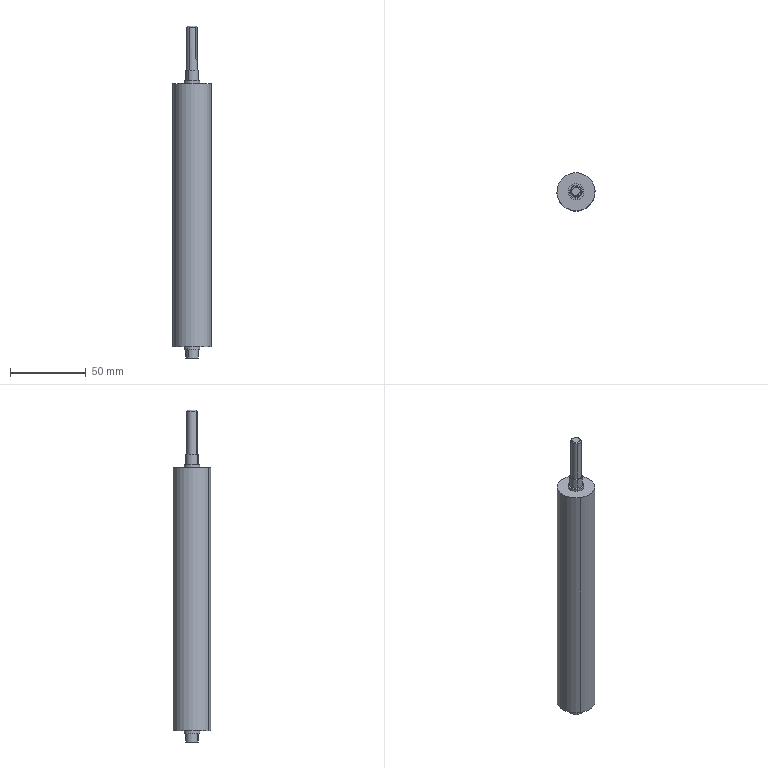Part | SolidWorks | features SplitBody 1 | 1 solid | 27 faces | box 25.2 x 25.2 x 219.8 mm | volume 89003 mm3 | cylinder 14 | plane 10 | cone 3 | commonest cylinder face diameters 8.4 x4 10.5 x4 2.1 x2 7 x2 25.2 x2
STEP:
#1=CARTESIAN_POINT('',(-72.98,240.467,-234.916));
#2=VERTEX_POINT('',#1);
#3=CARTESIAN_POINT('',(-69.853,240.613,-234.916));
#4=VERTEX_POINT('',#3);
#5=CARTESIAN_POINT('',(-71.525,242.859,-234.916));
#6=DIRECTION('',(0.,0.,1.));
#7=DIRECTION('',(-0.5199,-0.8543,0.));
#8=AXIS2_PLACEMENT_3D('',#5,#6,#7);
#9=CIRCLE('',#8,2.8);
#10=EDGE_CURVE('',#2,#4,#9,.T.);
#11=ORIENTED_EDGE('',*,*,#10,.F.);
#12=CARTESIAN_POINT('',(-73.344,239.869,-235.616));
#13=VERTEX_POINT('',#12);
#14=CARTESIAN_POINT('',(-72.98,240.467,-234.916));
#15=DIRECTION('',(-0.3676,-0.604,-0.7071));
#16=VECTOR('',#15,1000.);
#17=LINE('',#14,#16);
#18=EDGE_CURVE('',#2,#13,#17,.T.);
#19=ORIENTED_EDGE('',*,*,#18,.T.);
#20=CARTESIAN_POINT('',(-69.218,240.226,-235.616));
#21=VERTEX_POINT('',#20);
#22=CARTESIAN_POINT('',(-71.525,242.859,-235.616));
#23=DIRECTION('',(0.,0.,-1.));
#24=DIRECTION('',(-0.5199,-0.8543,0.));
#25=AXIS2_PLACEMENT_3D('',#22,#23,#24);
#26=CIRCLE('',#25,3.5);
#27=EDGE_CURVE('',#21,#13,#26,.T.);
#28=ORIENTED_EDGE('',*,*,#27,.F.);
#29=CARTESIAN_POINT('',(-69.853,240.613,-234.916));
#30=CARTESIAN_POINT('',(-69.64,240.483,-235.147));
#31=CARTESIAN_POINT('',(-69.429,240.354,-235.381));
#32=CARTESIAN_POINT('',(-69.218,240.226,-235.616));
#33=B_SPLINE_CURVE_WITH_KNOTS('',3,(#29,#30,#31,#32),.UNSPECIFIED.,.F.,.F.,(4,4),(0.,0.001021),.UNSPECIFIED.);
#34=EDGE_CURVE('',#4,#21,#33,.T.);
#35=ORIENTED_EDGE('',*,*,#34,.F.);
#36=EDGE_LOOP('',(#11,#19,#28,#35));
#37=FACE_OUTER_BOUND('',#36,.T.);
#38=CARTESIAN_POINT('',(-71.525,242.859,-234.916));
#39=DIRECTION('',(0.,0.,-1.));
#40=DIRECTION('',(0.5199,0.8543,0.));
#41=AXIS2_PLACEMENT_3D('',#38,#39,#40);
#42=CONICAL_SURFACE('',#41,2.8,0.7854);
#43=ADVANCED_FACE('',(#37),#42,.T.);
#44=ORIENTED_EDGE('',*,*,#18,.F.);
#45=CARTESIAN_POINT('',(-70.069,245.251,-234.916));
#46=VERTEX_POINT('',#45);
#47=CARTESIAN_POINT('',(-71.525,242.859,-234.916));
#48=DIRECTION('',(0.,0.,1.));
#49=DIRECTION('',(-0.5199,-0.8543,0.));
#50=AXIS2_PLACEMENT_3D('',#47,#48,#49);
#51=CIRCLE('',#50,2.8);
#52=EDGE_CURVE('',#46,#2,#51,.T.);
#53=ORIENTED_EDGE('',*,*,#52,.F.);
#54=CARTESIAN_POINT('',(-69.705,245.849,-235.616));
#55=VERTEX_POINT('',#54);
#56=CARTESIAN_POINT('',(-70.069,245.251,-234.916));
#57=DIRECTION('',(0.3676,0.604,-0.7071));
#58=VECTOR('',#57,1000.);
#59=LINE('',#56,#58);
#60=EDGE_CURVE('',#46,#55,#59,.T.);
#61=ORIENTED_EDGE('',*,*,#60,.T.);
#62=CARTESIAN_POINT('',(-71.525,242.859,-235.616));
#63=DIRECTION('',(0.,0.,-1.));
#64=DIRECTION('',(-0.5199,-0.8543,0.));
#65=AXIS2_PLACEMENT_3D('',#62,#63,#64);
#66=CIRCLE('',#65,3.5);
#67=EDGE_CURVE('',#13,#55,#66,.T.);
#68=ORIENTED_EDGE('',*,*,#67,.F.);
#69=EDGE_LOOP('',(#44,#53,#61,#68));
#70=FACE_OUTER_BOUND('',#69,.T.);
#71=CARTESIAN_POINT('',(-71.525,242.859,-234.916));
#72=DIRECTION('',(0.,0.,-1.));
#73=DIRECTION('',(0.5199,0.8543,0.));
#74=AXIS2_PLACEMENT_3D('',#71,#72,#73);
#75=CONICAL_SURFACE('',#74,2.8,0.7854);
#76=ADVANCED_FACE('',(#70),#75,.T.);
#77=CARTESIAN_POINT('',(-68.535,241.04,-256.966));
#78=VERTEX_POINT('',#77);
#79=CARTESIAN_POINT('',(-69.218,240.226,-255.916));
#80=VERTEX_POINT('',#79);
#81=CARTESIAN_POINT('',(-68.535,241.04,-256.966));
#82=CARTESIAN_POINT('',(-68.606,240.922,-256.966));
#83=CARTESIAN_POINT('',(-68.685,240.809,-256.938));
#84=CARTESIAN_POINT('',(-68.843,240.606,-256.832));
#85=CARTESIAN_POINT('',(-68.921,240.518,-256.755));
#86=CARTESIAN_POINT('',(-69.057,240.375,-256.561));
#87=CARTESIAN_POINT('',(-69.115,240.32,-256.445));
#88=CARTESIAN_POINT('',(-69.196,240.246,-256.193));
#89=CARTESIAN_POINT('',(-69.218,240.226,-256.055));
#90=CARTESIAN_POINT('',(-69.218,240.226,-255.916));
#91=B_SPLINE_CURVE_WITH_KNOTS('',3,(#81,#82,#83,#84,#85,#86,#87,#88,#89,#90),.UNSPECIFIED.,.F.,.F.,(4,2,2,2,4),(0.001651,0.002064,0.002476,0.002888,0.003301),.UNSPECIFIED.);
#92=EDGE_CURVE('',#78,#80,#91,.T.);
#93=ORIENTED_EDGE('',*,*,#92,.F.);
#94=CARTESIAN_POINT('',(-69.671,241.731,-256.966));
#95=VERTEX_POINT('',#94);
#96=CARTESIAN_POINT('',(-60.761,236.309,-256.966));
#97=DIRECTION('',(-0.8543,0.5199,0.));
#98=VECTOR('',#97,1000.);
#99=LINE('',#96,#98);
#100=EDGE_CURVE('',#78,#95,#99,.T.);
#101=ORIENTED_EDGE('',*,*,#100,.T.);
#102=CARTESIAN_POINT('',(-70.217,240.834,-255.916));
#103=VERTEX_POINT('',#102);
#104=CARTESIAN_POINT('',(-69.671,241.731,-255.916));
#105=DIRECTION('',(0.8543,-0.5199,0.));
#106=DIRECTION('',(0.,0.,-1.));
#107=AXIS2_PLACEMENT_3D('',#104,#105,#106);
#108=CIRCLE('',#107,1.05);
#109=EDGE_CURVE('',#103,#95,#108,.T.);
#110=ORIENTED_EDGE('',*,*,#109,.F.);
#111=CARTESIAN_POINT('',(-61.307,235.412,-255.916));
#112=DIRECTION('',(-0.8543,0.5199,0.));
#113=VECTOR('',#112,1000.);
#114=LINE('',#111,#113);
#115=EDGE_CURVE('',#80,#103,#114,.T.);
#116=ORIENTED_EDGE('',*,*,#115,.F.);
#117=EDGE_LOOP('',(#93,#101,#110,#116));
#118=FACE_OUTER_BOUND('',#117,.T.);
#119=CARTESIAN_POINT('',(-60.761,236.309,-255.916));
#120=DIRECTION('',(-0.8543,0.5199,0.));
#121=DIRECTION('',(0.,0.,-1.));
#122=AXIS2_PLACEMENT_3D('',#119,#120,#121);
#123=CYLINDRICAL_SURFACE('',#122,1.05);
#124=ADVANCED_FACE('',(#118),#123,.F.);
#125=CARTESIAN_POINT('',(-69.341,246.447,-454.716));
#126=VERTEX_POINT('',#125);
#127=CARTESIAN_POINT('',(-73.708,239.271,-454.716));
#128=VERTEX_POINT('',#127);
#129=CARTESIAN_POINT('',(-71.525,242.859,-454.716));
#130=DIRECTION('',(0.,0.,-1.));
#131=DIRECTION('',(0.5199,0.8543,0.));
#132=AXIS2_PLACEMENT_3D('',#129,#130,#131);
#133=CIRCLE('',#132,4.2);
#134=EDGE_CURVE('',#126,#128,#133,.T.);
#135=ORIENTED_EDGE('',*,*,#134,.F.);
#136=CARTESIAN_POINT('',(-69.341,246.447,-449.116));
#137=VERTEX_POINT('',#136);
#138=CARTESIAN_POINT('',(-69.341,246.447,-454.716));
#139=DIRECTION('',(0.,0.,1.));
#140=VECTOR('',#139,1000.);
#141=LINE('',#138,#140);
#142=EDGE_CURVE('',#126,#137,#141,.T.);
#143=ORIENTED_EDGE('',*,*,#142,.T.);
#144=CARTESIAN_POINT('',(-73.708,239.271,-449.116));
#145=VERTEX_POINT('',#144);
#146=CARTESIAN_POINT('',(-71.525,242.859,-449.116));
#147=DIRECTION('',(0.,0.,-1.));
#148=DIRECTION('',(0.5199,0.8543,0.));
#149=AXIS2_PLACEMENT_3D('',#146,#147,#148);
#150=CIRCLE('',#149,4.2);
#151=EDGE_CURVE('',#137,#145,#150,.T.);
#152=ORIENTED_EDGE('',*,*,#151,.T.);
#153=CARTESIAN_POINT('',(-73.708,239.271,-454.716));
#154=DIRECTION('',(0.,0.,1.));
#155=VECTOR('',#154,1000.);
#156=LINE('',#153,#155);
#157=EDGE_CURVE('',#128,#145,#156,.T.);
#158=ORIENTED_EDGE('',*,*,#157,.F.);
#159=EDGE_LOOP('',(#135,#143,#152,#158));
#160=FACE_OUTER_BOUND('',#159,.T.);
#161=CARTESIAN_POINT('',(-71.525,242.859,-454.716));
#162=DIRECTION('',(0.,0.,1.));
#163=DIRECTION('',(-0.5199,-0.8543,0.));
#164=AXIS2_PLACEMENT_3D('',#161,#162,#163);
#165=CYLINDRICAL_SURFACE('',#164,4.2);
#166=ADVANCED_FACE('',(#160),#165,.T.);
#167=CARTESIAN_POINT('',(-73.708,239.271,-264.316));
#168=VERTEX_POINT('',#167);
#169=CARTESIAN_POINT('',(-69.341,246.447,-264.316));
#170=VERTEX_POINT('',#169);
#171=CARTESIAN_POINT('',(-71.525,242.859,-264.316));
#172=DIRECTION('',(0.,0.,1.));
#173=DIRECTION('',(-0.5199,-0.8543,0.));
#174=AXIS2_PLACEMENT_3D('',#171,#172,#173);
#175=CIRCLE('',#174,4.2);
#176=EDGE_CURVE('',#168,#170,#175,.T.);
#177=ORIENTED_EDGE('',*,*,#176,.F.);
#178=CARTESIAN_POINT('',(-73.708,239.271,-271.316));
#179=VERTEX_POINT('',#178);
#180=CARTESIAN_POINT('',(-73.708,239.271,-264.316));
#181=DIRECTION('',(0.,0.,-1.));
#182=VECTOR('',#181,1000.);
#183=LINE('',#180,#182);
#184=EDGE_CURVE('',#168,#179,#183,.T.);
#185=ORIENTED_EDGE('',*,*,#184,.T.);
#186=CARTESIAN_POINT('',(-69.341,246.447,-271.316));
#187=VERTEX_POINT('',#186);
#188=CARTESIAN_POINT('',(-71.525,242.859,-271.316));
#189=DIRECTION('',(0.,0.,1.));
#190=DIRECTION('',(-0.5199,-0.8543,0.));
#191=AXIS2_PLACEMENT_3D('',#188,#189,#190);
#192=CIRCLE('',#191,4.2);
#193=EDGE_CURVE('',#179,#187,#192,.T.);
#194=ORIENTED_EDGE('',*,*,#193,.T.);
#195=CARTESIAN_POINT('',(-69.341,246.447,-264.316));
#196=DIRECTION('',(0.,0.,-1.));
#197=VECTOR('',#196,1000.);
#198=LINE('',#195,#197);
#199=EDGE_CURVE('',#170,#187,#198,.T.);
#200=ORIENTED_EDGE('',*,*,#199,.F.);
#201=EDGE_LOOP('',(#177,#185,#194,#200));
#202=FACE_OUTER_BOUND('',#201,.T.);
#203=CARTESIAN_POINT('',(-71.525,242.859,-264.316));
#204=DIRECTION('',(0.,0.,-1.));
#205=DIRECTION('',(0.5199,0.8543,0.));
#206=AXIS2_PLACEMENT_3D('',#203,#204,#205);
#207=CYLINDRICAL_SURFACE('',#206,4.2);
#208=ADVANCED_FACE('',(#202),#207,.T.);
#209=CARTESIAN_POINT('',(-68.795,247.344,-449.116));
#210=VERTEX_POINT('',#209);
#211=CARTESIAN_POINT('',(-74.254,238.374,-449.116));
#212=VERTEX_POINT('',#211);
#213=CARTESIAN_POINT('',(-71.525,242.859,-449.116));
#214=DIRECTION('',(0.,0.,-1.));
#215=DIRECTION('',(0.5199,0.8543,0.));
#216=AXIS2_PLACEMENT_3D('',#213,#214,#215);
#217=CIRCLE('',#216,5.25);
#218=EDGE_CURVE('',#210,#212,#217,.T.);
#219=ORIENTED_EDGE('',*,*,#218,.F.);
#220=CARTESIAN_POINT('',(-68.795,247.344,-447.366));
#221=VERTEX_POINT('',#220);
#222=CARTESIAN_POINT('',(-68.795,247.344,-449.116));
#223=DIRECTION('',(0.,0.,1.));
#224=VECTOR('',#223,1000.);
#225=LINE('',#222,#224);
#226=EDGE_CURVE('',#210,#221,#225,.T.);
#227=ORIENTED_EDGE('',*,*,#226,.T.);
#228=CARTESIAN_POINT('',(-74.254,238.374,-447.366));
#229=VERTEX_POINT('',#228);
#230=CARTESIAN_POINT('',(-71.525,242.859,-447.366));
#231=DIRECTION('',(0.,0.,-1.));
#232=DIRECTION('',(-0.5199,-0.8543,0.));
#233=AXIS2_PLACEMENT_3D('',#230,#231,#232);
#234=CIRCLE('',#233,5.25);
#235=EDGE_CURVE('',#221,#229,#234,.T.);
#236=ORIENTED_EDGE('',*,*,#235,.T.);
#237=CARTESIAN_POINT('',(-74.254,238.374,-449.116));
#238=DIRECTION('',(0.,0.,1.));
#239=VECTOR('',#238,1000.);
#240=LINE('',#237,#239);
#241=EDGE_CURVE('',#212,#229,#240,.T.);
#242=ORIENTED_EDGE('',*,*,#241,.F.);
#243=EDGE_LOOP('',(#219,#227,#236,#242));
#244=FACE_OUTER_BOUND('',#243,.T.);
#245=CARTESIAN_POINT('',(-71.525,242.859,-449.116));
#246=DIRECTION('',(0.,0.,1.));
#247=DIRECTION('',(-0.5199,-0.8543,0.));
#248=AXIS2_PLACEMENT_3D('',#245,#246,#247);
#249=CYLINDRICAL_SURFACE('',#248,5.25);
#250=ADVANCED_FACE('',(#244),#249,.T.);
#251=CARTESIAN_POINT('',(-74.254,238.374,-271.316));
#252=VERTEX_POINT('',#251);
#253=CARTESIAN_POINT('',(-68.795,247.344,-271.316));
#254=VERTEX_POINT('',#253);
#255=CARTESIAN_POINT('',(-71.525,242.859,-271.316));
#256=DIRECTION('',(0.,0.,1.));
#257=DIRECTION('',(-0.5199,-0.8543,0.));
#258=AXIS2_PLACEMENT_3D('',#255,#256,#257);
#259=CIRCLE('',#258,5.25);
#260=EDGE_CURVE('',#252,#254,#259,.T.);
#261=ORIENTED_EDGE('',*,*,#260,.F.);
#262=CARTESIAN_POINT('',(-74.254,238.374,-273.066));
#263=VERTEX_POINT('',#262);
#264=CARTESIAN_POINT('',(-74.254,238.374,-271.316));
#265=DIRECTION('',(0.,0.,-1.));
#266=VECTOR('',#265,1000.);
#267=LINE('',#264,#266);
#268=EDGE_CURVE('',#252,#263,#267,.T.);
#269=ORIENTED_EDGE('',*,*,#268,.T.);
#270=CARTESIAN_POINT('',(-68.795,247.344,-273.066));
#271=VERTEX_POINT('',#270);
#272=CARTESIAN_POINT('',(-71.525,242.859,-273.066));
#273=DIRECTION('',(0.,0.,1.));
#274=DIRECTION('',(-0.5199,-0.8543,0.));
#275=AXIS2_PLACEMENT_3D('',#272,#273,#274);
#276=CIRCLE('',#275,5.25);
#277=EDGE_CURVE('',#263,#271,#276,.T.);
#278=ORIENTED_EDGE('',*,*,#277,.T.);
#279=CARTESIAN_POINT('',(-68.795,247.344,-271.316));
#280=DIRECTION('',(0.,0.,-1.));
#281=VECTOR('',#280,1000.);
#282=LINE('',#279,#281);
#283=EDGE_CURVE('',#254,#271,#282,.T.);
#284=ORIENTED_EDGE('',*,*,#283,.F.);
#285=EDGE_LOOP('',(#261,#269,#278,#284));
#286=FACE_OUTER_BOUND('',#285,.T.);
#287=CARTESIAN_POINT('',(-71.525,242.859,-271.316));
#288=DIRECTION('',(0.,0.,-1.));
#289=DIRECTION('',(0.5199,0.8543,0.));
#290=AXIS2_PLACEMENT_3D('',#287,#288,#289);
#291=CYLINDRICAL_SURFACE('',#290,5.25);
#292=ADVANCED_FACE('',(#286),#291,.T.);
#293=CARTESIAN_POINT('',(-78.075,232.095,-273.066));
#294=VERTEX_POINT('',#293);
#295=CARTESIAN_POINT('',(-64.975,253.623,-273.066));
#296=VERTEX_POINT('',#295);
#297=CARTESIAN_POINT('',(-71.525,242.859,-273.066));
#298=DIRECTION('',(0.,0.,1.));
#299=DIRECTION('',(-0.5199,-0.8543,0.));
#300=AXIS2_PLACEMENT_3D('',#297,#298,#299);
#301=CIRCLE('',#300,12.6);
#302=EDGE_CURVE('',#294,#296,#301,.T.);
#303=ORIENTED_EDGE('',*,*,#302,.F.);
#304=CARTESIAN_POINT('',(-78.075,232.095,-447.366));
#305=VERTEX_POINT('',#304);
#306=CARTESIAN_POINT('',(-78.075,232.095,-273.066));
#307=DIRECTION('',(0.,0.,-1.));
#308=VECTOR('',#307,1000.);
#309=LINE('',#306,#308);
#310=EDGE_CURVE('',#294,#305,#309,.T.);
#311=ORIENTED_EDGE('',*,*,#310,.T.);
#312=CARTESIAN_POINT('',(-64.975,253.623,-447.366));
#313=VERTEX_POINT('',#312);
#314=CARTESIAN_POINT('',(-71.525,242.859,-447.366));
#315=DIRECTION('',(0.,0.,1.));
#316=DIRECTION('',(-0.5199,-0.8543,0.));
#317=AXIS2_PLACEMENT_3D('',#314,#315,#316);
#318=CIRCLE('',#317,12.6);
#319=EDGE_CURVE('',#305,#313,#318,.T.);
#320=ORIENTED_EDGE('',*,*,#319,.T.);
#321=CARTESIAN_POINT('',(-64.975,253.623,-273.066));
#322=DIRECTION('',(0.,0.,-1.));
#323=VECTOR('',#322,1000.);
#324=LINE('',#321,#323);
#325=EDGE_CURVE('',#296,#313,#324,.T.);
#326=ORIENTED_EDGE('',*,*,#325,.F.);
#327=EDGE_LOOP('',(#303,#311,#320,#326));
#328=FACE_OUTER_BOUND('',#327,.T.);
#329=CARTESIAN_POINT('',(-71.525,242.859,-273.066));
#330=DIRECTION('',(0.,0.,-1.));
#331=DIRECTION('',(0.5199,0.8543,0.));
#332=AXIS2_PLACEMENT_3D('',#329,#330,#331);
#333=CYLINDRICAL_SURFACE('',#332,12.6);
#334=ADVANCED_FACE('',(#328),#333,.T.);
#335=ORIENTED_EDGE('',*,*,#27,.T.);
#336=CARTESIAN_POINT('',(-73.344,239.869,-264.316));
#337=VERTEX_POINT('',#336);
#338=CARTESIAN_POINT('',(-73.344,239.869,-241.916));
#339=DIRECTION('',(0.,0.,-1.));
#340=VECTOR('',#339,1000.);
#341=LINE('',#338,#340);
#342=EDGE_CURVE('',#13,#337,#341,.T.);
#343=ORIENTED_EDGE('',*,*,#342,.T.);
#344=CARTESIAN_POINT('',(-69.705,245.849,-264.316));
#345=VERTEX_POINT('',#344);
#346=CARTESIAN_POINT('',(-71.525,242.859,-264.316));
#347=DIRECTION('',(0.,0.,1.));
#348=DIRECTION('',(-0.5199,-0.8543,0.));
#349=AXIS2_PLACEMENT_3D('',#346,#347,#348);
#350=CIRCLE('',#349,3.5);
#351=EDGE_CURVE('',#337,#345,#350,.T.);
#352=ORIENTED_EDGE('',*,*,#351,.T.);
#353=CARTESIAN_POINT('',(-69.705,245.849,-241.916));
#354=DIRECTION('',(0.,0.,-1.));
#355=VECTOR('',#354,1000.);
#356=LINE('',#353,#355);
#357=EDGE_CURVE('',#55,#345,#356,.T.);
#358=ORIENTED_EDGE('',*,*,#357,.F.);
#359=CARTESIAN_POINT('',(-68.127,242.02,-235.616));
#360=VERTEX_POINT('',#359);
#361=CARTESIAN_POINT('',(-71.525,242.859,-235.616));
#362=DIRECTION('',(0.,0.,-1.));
#363=DIRECTION('',(-0.5199,-0.8543,0.));
#364=AXIS2_PLACEMENT_3D('',#361,#362,#363);
#365=CIRCLE('',#364,3.5);
#366=EDGE_CURVE('',#55,#360,#365,.T.);
#367=ORIENTED_EDGE('',*,*,#366,.T.);
#368=CARTESIAN_POINT('',(-68.127,242.02,-255.916));
#369=VERTEX_POINT('',#368);
#370=CARTESIAN_POINT('',(-68.127,242.02,-241.916));
#371=DIRECTION('',(0.,0.,-1.));
#372=VECTOR('',#371,1000.);
#373=LINE('',#370,#372);
#374=EDGE_CURVE('',#360,#369,#373,.T.);
#375=ORIENTED_EDGE('',*,*,#374,.T.);
#376=CARTESIAN_POINT('',(-68.127,242.02,-255.916));
#377=CARTESIAN_POINT('',(-68.127,242.02,-256.055));
#378=CARTESIAN_POINT('',(-68.133,241.992,-256.192));
#379=CARTESIAN_POINT('',(-68.162,241.886,-256.446));
#380=CARTESIAN_POINT('',(-68.185,241.808,-256.562));
#381=CARTESIAN_POINT('',(-68.249,241.622,-256.755));
#382=CARTESIAN_POINT('',(-68.292,241.511,-256.833));
#383=CARTESIAN_POINT('',(-68.398,241.28,-256.938));
#384=CARTESIAN_POINT('',(-68.463,241.157,-256.966));
#385=CARTESIAN_POINT('',(-68.535,241.04,-256.966));
#386=B_SPLINE_CURVE_WITH_KNOTS('',3,(#376,#377,#378,#379,#380,#381,#382,#383,#384,#385),.UNSPECIFIED.,.F.,.F.,(4,2,2,2,4),(0.,0.0004128,0.0008257,0.001239,0.001651),.UNSPECIFIED.);
#387=EDGE_CURVE('',#369,#78,#386,.T.);
#388=ORIENTED_EDGE('',*,*,#387,.T.);
#389=ORIENTED_EDGE('',*,*,#92,.T.);
#390=CARTESIAN_POINT('',(-69.218,240.226,-241.916));
#391=DIRECTION('',(0.,0.,1.));
#392=VECTOR('',#391,1000.);
#393=LINE('',#390,#392);
#394=EDGE_CURVE('',#80,#21,#393,.T.);
#395=ORIENTED_EDGE('',*,*,#394,.T.);
#396=EDGE_LOOP('',(#335,#343,#352,#358,#367,#375,#388,#389,#395));
#397=FACE_OUTER_BOUND('',#396,.T.);
#398=CARTESIAN_POINT('',(-71.525,242.859,-241.916));
#399=DIRECTION('',(0.,0.,-1.));
#400=DIRECTION('',(0.5199,0.8543,0.));
#401=AXIS2_PLACEMENT_3D('',#398,#399,#400);
#402=CYLINDRICAL_SURFACE('',#401,3.5);
#403=ADVANCED_FACE('',(#397),#402,.T.);
#404=ORIENTED_EDGE('',*,*,#342,.F.);
#405=ORIENTED_EDGE('',*,*,#67,.T.);
#406=ORIENTED_EDGE('',*,*,#357,.T.);
#407=CARTESIAN_POINT('',(-71.525,242.859,-264.316));
#408=DIRECTION('',(0.,0.,1.));
#409=DIRECTION('',(-0.5199,-0.8543,0.));
#410=AXIS2_PLACEMENT_3D('',#407,#408,#409);
#411=CIRCLE('',#410,3.5);
#412=EDGE_CURVE('',#345,#337,#411,.T.);
#413=ORIENTED_EDGE('',*,*,#412,.T.);
#414=EDGE_LOOP('',(#404,#405,#406,#413));
#415=FACE_OUTER_BOUND('',#414,.T.);
#416=CARTESIAN_POINT('',(-71.525,242.859,-241.916));
#417=DIRECTION('',(0.,0.,-1.));
#418=DIRECTION('',(0.5199,0.8543,0.));
#419=AXIS2_PLACEMENT_3D('',#416,#417,#418);
#420=CYLINDRICAL_SURFACE('',#419,3.5);
#421=ADVANCED_FACE('',(#415),#420,.T.);
#422=CARTESIAN_POINT('',(-71.525,242.859,-449.116));
#423=DIRECTION('',(0.,0.,-1.));
#424=DIRECTION('',(0.5199,0.8543,0.));
#425=AXIS2_PLACEMENT_3D('',#422,#423,#424);
#426=CIRCLE('',#425,5.25);
#427=EDGE_CURVE('',#212,#210,#426,.T.);
#428=ORIENTED_EDGE('',*,*,#427,.T.);
#429=ORIENTED_EDGE('',*,*,#218,.T.);
#430=EDGE_LOOP('',(#428,#429));
#431=FACE_OUTER_BOUND('',#430,.T.);
#432=CARTESIAN_POINT('',(-71.525,242.859,-449.116));
#433=DIRECTION('',(0.,0.,-1.));
#434=DIRECTION('',(0.5199,0.8543,0.));
#435=AXIS2_PLACEMENT_3D('',#432,#433,#434);
#436=CIRCLE('',#435,4.2);
#437=EDGE_CURVE('',#145,#137,#436,.T.);
#438=ORIENTED_EDGE('',*,*,#437,.F.);
#439=ORIENTED_EDGE('',*,*,#151,.F.);
#440=EDGE_LOOP('',(#438,#439));
#441=FACE_BOUND('',#440,.T.);
#442=CARTESIAN_POINT('',(-71.525,242.859,-449.116));
#443=DIRECTION('',(0.,0.,-1.));
#444=DIRECTION('',(0.5199,0.8543,0.));
#445=AXIS2_PLACEMENT_3D('',#442,#443,#444);
#446=PLANE('',#445);
#447=ADVANCED_FACE('',(#431,#441),#446,.T.);
#448=CARTESIAN_POINT('',(-71.525,242.859,-271.316));
#449=DIRECTION('',(0.,0.,1.));
#450=DIRECTION('',(-0.5199,-0.8543,0.));
#451=AXIS2_PLACEMENT_3D('',#448,#449,#450);
#452=CIRCLE('',#451,5.25);
#453=EDGE_CURVE('',#254,#252,#452,.T.);
#454=ORIENTED_EDGE('',*,*,#453,.T.);
#455=ORIENTED_EDGE('',*,*,#260,.T.);
#456=EDGE_LOOP('',(#454,#455));
#457=FACE_OUTER_BOUND('',#456,.T.);
#458=CARTESIAN_POINT('',(-71.525,242.859,-271.316));
#459=DIRECTION('',(0.,0.,1.));
#460=DIRECTION('',(-0.5199,-0.8543,0.));
#461=AXIS2_PLACEMENT_3D('',#458,#459,#460);
#462=CIRCLE('',#461,4.2);
#463=EDGE_CURVE('',#187,#179,#462,.T.);
#464=ORIENTED_EDGE('',*,*,#463,.F.);
#465=ORIENTED_EDGE('',*,*,#193,.F.);
#466=EDGE_LOOP('',(#464,#465));
#467=FACE_BOUND('',#466,.T.);
#468=CARTESIAN_POINT('',(-71.525,242.859,-271.316));
#469=DIRECTION('',(0.,0.,1.));
#470=DIRECTION('',(-0.5199,-0.8543,0.));
#471=AXIS2_PLACEMENT_3D('',#468,#469,#470);
#472=PLANE('',#471);
#473=ADVANCED_FACE('',(#457,#467),#472,.T.);
#474=CARTESIAN_POINT('',(-71.525,242.859,-447.366));
#475=DIRECTION('',(0.,0.,1.));
#476=DIRECTION('',(-0.5199,-0.8543,0.));
#477=AXIS2_PLACEMENT_3D('',#474,#475,#476);
#478=CIRCLE('',#477,12.6);
#479=EDGE_CURVE('',#313,#305,#478,.T.);
#480=ORIENTED_EDGE('',*,*,#479,.F.);
#481=ORIENTED_EDGE('',*,*,#319,.F.);
#482=EDGE_LOOP('',(#480,#481));
#483=FACE_OUTER_BOUND('',#482,.T.);
#484=CARTESIAN_POINT('',(-71.525,242.859,-447.366));
#485=DIRECTION('',(0.,0.,-1.));
#486=DIRECTION('',(-0.5199,-0.8543,0.));
#487=AXIS2_PLACEMENT_3D('',#484,#485,#486);
#488=CIRCLE('',#487,5.25);
#489=EDGE_CURVE('',#229,#221,#488,.T.);
#490=ORIENTED_EDGE('',*,*,#489,.F.);
#491=ORIENTED_EDGE('',*,*,#235,.F.);
#492=EDGE_LOOP('',(#490,#491));
#493=FACE_BOUND('',#492,.T.);
#494=CARTESIAN_POINT('',(-71.525,242.859,-447.366));
#495=DIRECTION('',(0.,0.,1.));
#496=DIRECTION('',(-0.5199,-0.8543,0.));
#497=AXIS2_PLACEMENT_3D('',#494,#495,#496);
#498=PLANE('',#497);
#499=ADVANCED_FACE('',(#483,#493),#498,.F.);
#500=CARTESIAN_POINT('',(-71.525,242.859,-273.066));
#501=DIRECTION('',(0.,0.,1.));
#502=DIRECTION('',(-0.5199,-0.8543,0.));
#503=AXIS2_PLACEMENT_3D('',#500,#501,#502);
#504=CIRCLE('',#503,12.6);
#505=EDGE_CURVE('',#296,#294,#504,.T.);
#506=ORIENTED_EDGE('',*,*,#505,.T.);
#507=ORIENTED_EDGE('',*,*,#302,.T.);
#508=EDGE_LOOP('',(#506,#507));
#509=FACE_OUTER_BOUND('',#508,.T.);
#510=CARTESIAN_POINT('',(-71.525,242.859,-273.066));
#511=DIRECTION('',(0.,0.,1.));
#512=DIRECTION('',(-0.5199,-0.8543,0.));
#513=AXIS2_PLACEMENT_3D('',#510,#511,#512);
#514=CIRCLE('',#513,5.25);
#515=EDGE_CURVE('',#271,#263,#514,.T.);
#516=ORIENTED_EDGE('',*,*,#515,.F.);
#517=ORIENTED_EDGE('',*,*,#277,.F.);
#518=EDGE_LOOP('',(#516,#517));
#519=FACE_BOUND('',#518,.T.);
#520=CARTESIAN_POINT('',(-71.525,242.859,-273.066));
#521=DIRECTION('',(0.,0.,1.));
#522=DIRECTION('',(-0.5199,-0.8543,0.));
#523=AXIS2_PLACEMENT_3D('',#520,#521,#522);
#524=PLANE('',#523);
#525=ADVANCED_FACE('',(#509,#519),#524,.T.);
#526=ORIENTED_EDGE('',*,*,#310,.F.);
#527=ORIENTED_EDGE('',*,*,#505,.F.);
#528=ORIENTED_EDGE('',*,*,#325,.T.);
#529=ORIENTED_EDGE('',*,*,#479,.T.);
#530=EDGE_LOOP('',(#526,#527,#528,#529));
#531=FACE_OUTER_BOUND('',#530,.T.);
#532=CARTESIAN_POINT('',(-71.525,242.859,-273.066));
#533=DIRECTION('',(0.,0.,-1.));
#534=DIRECTION('',(0.5199,0.8543,0.));
#535=AXIS2_PLACEMENT_3D('',#532,#533,#534);
#536=CYLINDRICAL_SURFACE('',#535,12.6);
#537=ADVANCED_FACE('',(#531),#536,.T.);
#538=ORIENTED_EDGE('',*,*,#268,.F.);
#539=ORIENTED_EDGE('',*,*,#453,.F.);
#540=ORIENTED_EDGE('',*,*,#283,.T.);
#541=ORIENTED_EDGE('',*,*,#515,.T.);
#542=EDGE_LOOP('',(#538,#539,#540,#541));
#543=FACE_OUTER_BOUND('',#542,.T.);
#544=CARTESIAN_POINT('',(-71.525,242.859,-271.316));
#545=DIRECTION('',(0.,0.,-1.));
#546=DIRECTION('',(0.5199,0.8543,0.));
#547=AXIS2_PLACEMENT_3D('',#544,#545,#546);
#548=CYLINDRICAL_SURFACE('',#547,5.25);
#549=ADVANCED_FACE('',(#543),#548,.T.);
#550=ORIENTED_EDGE('',*,*,#226,.F.);
#551=ORIENTED_EDGE('',*,*,#427,.F.);
#552=ORIENTED_EDGE('',*,*,#241,.T.);
#553=ORIENTED_EDGE('',*,*,#489,.T.);
#554=EDGE_LOOP('',(#550,#551,#552,#553));
#555=FACE_OUTER_BOUND('',#554,.T.);
#556=CARTESIAN_POINT('',(-71.525,242.859,-449.116));
#557=DIRECTION('',(0.,0.,1.));
#558=DIRECTION('',(-0.5199,-0.8543,0.));
#559=AXIS2_PLACEMENT_3D('',#556,#557,#558);
#560=CYLINDRICAL_SURFACE('',#559,5.25);
#561=ADVANCED_FACE('',(#555),#560,.T.);
#562=ORIENTED_EDGE('',*,*,#184,.F.);
#563=CARTESIAN_POINT('',(-71.525,242.859,-264.316));
#564=DIRECTION('',(0.,0.,1.));
#565=DIRECTION('',(-0.5199,-0.8543,0.));
#566=AXIS2_PLACEMENT_3D('',#563,#564,#565);
#567=CIRCLE('',#566,4.2);
#568=EDGE_CURVE('',#170,#168,#567,.T.);
#569=ORIENTED_EDGE('',*,*,#568,.F.);
#570=ORIENTED_EDGE('',*,*,#199,.T.);
#571=ORIENTED_EDGE('',*,*,#463,.T.);
#572=EDGE_LOOP('',(#562,#569,#570,#571));
#573=FACE_OUTER_BOUND('',#572,.T.);
#574=CARTESIAN_POINT('',(-71.525,242.859,-264.316));
#575=DIRECTION('',(0.,0.,-1.));
#576=DIRECTION('',(0.5199,0.8543,0.));
#577=AXIS2_PLACEMENT_3D('',#574,#575,#576);
#578=CYLINDRICAL_SURFACE('',#577,4.2);
#579=ADVANCED_FACE('',(#573),#578,.T.);
#580=ORIENTED_EDGE('',*,*,#412,.F.);
#581=ORIENTED_EDGE('',*,*,#351,.F.);
#582=EDGE_LOOP('',(#580,#581));
#583=FACE_BOUND('',#582,.T.);
#584=ORIENTED_EDGE('',*,*,#568,.T.);
#585=ORIENTED_EDGE('',*,*,#176,.T.);
#586=EDGE_LOOP('',(#584,#585));
#587=FACE_OUTER_BOUND('',#586,.T.);
#588=CARTESIAN_POINT('',(-71.525,242.859,-264.316));
#589=DIRECTION('',(0.,0.,1.));
#590=DIRECTION('',(-0.5199,-0.8543,0.));
#591=AXIS2_PLACEMENT_3D('',#588,#589,#590);
#592=PLANE('',#591);
#593=ADVANCED_FACE('',(#583,#587),#592,.T.);
#594=ORIENTED_EDGE('',*,*,#142,.F.);
#595=CARTESIAN_POINT('',(-71.525,242.859,-454.716));
#596=DIRECTION('',(0.,0.,-1.));
#597=DIRECTION('',(0.5199,0.8543,0.));
#598=AXIS2_PLACEMENT_3D('',#595,#596,#597);
#599=CIRCLE('',#598,4.2);
#600=EDGE_CURVE('',#128,#126,#599,.T.);
#601=ORIENTED_EDGE('',*,*,#600,.F.);
#602=ORIENTED_EDGE('',*,*,#157,.T.);
#603=ORIENTED_EDGE('',*,*,#437,.T.);
#604=EDGE_LOOP('',(#594,#601,#602,#603));
#605=FACE_OUTER_BOUND('',#604,.T.);
#606=CARTESIAN_POINT('',(-71.525,242.859,-454.716));
#607=DIRECTION('',(0.,0.,1.));
#608=DIRECTION('',(-0.5199,-0.8543,0.));
#609=AXIS2_PLACEMENT_3D('',#606,#607,#608);
#610=CYLINDRICAL_SURFACE('',#609,4.2);
#611=ADVANCED_FACE('',(#605),#610,.T.);
#612=ORIENTED_EDGE('',*,*,#600,.T.);
#613=ORIENTED_EDGE('',*,*,#134,.T.);
#614=EDGE_LOOP('',(#612,#613));
#615=FACE_OUTER_BOUND('',#614,.T.);
#616=CARTESIAN_POINT('',(-71.525,242.859,-454.716));
#617=DIRECTION('',(0.,0.,-1.));
#618=DIRECTION('',(0.5199,0.8543,0.));
#619=AXIS2_PLACEMENT_3D('',#616,#617,#618);
#620=PLANE('',#619);
#621=ADVANCED_FACE('',(#615),#620,.T.);
#622=CARTESIAN_POINT('',(-70.217,240.834,-234.916));
#623=VERTEX_POINT('',#622);
#624=CARTESIAN_POINT('',(-70.217,240.834,-234.916));
#625=DIRECTION('',(-0.8543,0.5199,0.));
#626=VECTOR('',#625,1000.);
#627=LINE('',#624,#626);
#628=EDGE_CURVE('',#4,#623,#627,.T.);
#629=ORIENTED_EDGE('',*,*,#628,.F.);
#630=ORIENTED_EDGE('',*,*,#34,.T.);
#631=ORIENTED_EDGE('',*,*,#394,.F.);
#632=ORIENTED_EDGE('',*,*,#115,.T.);
#633=CARTESIAN_POINT('',(-70.217,240.834,-255.916));
#634=DIRECTION('',(0.,0.,-1.));
#635=VECTOR('',#634,1000.);
#636=LINE('',#633,#635);
#637=EDGE_CURVE('',#623,#103,#636,.T.);
#638=ORIENTED_EDGE('',*,*,#637,.F.);
#639=EDGE_LOOP('',(#629,#630,#631,#632,#638));
#640=FACE_OUTER_BOUND('',#639,.T.);
#641=CARTESIAN_POINT('',(-61.307,235.412,-255.916));
#642=DIRECTION('',(0.5199,0.8543,0.));
#643=DIRECTION('',(0.,0.,1.));
#644=AXIS2_PLACEMENT_3D('',#641,#642,#643);
#645=PLANE('',#644);
#646=ADVANCED_FACE('',(#640),#645,.T.);
#647=ORIENTED_EDGE('',*,*,#100,.F.);
#648=ORIENTED_EDGE('',*,*,#387,.F.);
#649=CARTESIAN_POINT('',(-69.125,242.628,-255.916));
#650=VERTEX_POINT('',#649);
#651=CARTESIAN_POINT('',(-60.215,237.206,-255.916));
#652=DIRECTION('',(-0.8543,0.5199,0.));
#653=VECTOR('',#652,1000.);
#654=LINE('',#651,#653);
#655=EDGE_CURVE('',#369,#650,#654,.T.);
#656=ORIENTED_EDGE('',*,*,#655,.T.);
#657=CARTESIAN_POINT('',(-69.671,241.731,-255.916));
#658=DIRECTION('',(0.8543,-0.5199,0.));
#659=DIRECTION('',(0.,0.,-1.));
#660=AXIS2_PLACEMENT_3D('',#657,#658,#659);
#661=CIRCLE('',#660,1.05);
#662=EDGE_CURVE('',#95,#650,#661,.T.);
#663=ORIENTED_EDGE('',*,*,#662,.F.);
#664=EDGE_LOOP('',(#647,#648,#656,#663));
#665=FACE_OUTER_BOUND('',#664,.T.);
#666=CARTESIAN_POINT('',(-60.761,236.309,-255.916));
#667=DIRECTION('',(-0.8543,0.5199,0.));
#668=DIRECTION('',(0.,0.,-1.));
#669=AXIS2_PLACEMENT_3D('',#666,#667,#668);
#670=CYLINDRICAL_SURFACE('',#669,1.05);
#671=ADVANCED_FACE('',(#665),#670,.F.);
#672=ORIENTED_EDGE('',*,*,#374,.F.);
#673=CARTESIAN_POINT('',(-68.761,242.407,-234.916));
#674=VERTEX_POINT('',#673);
#675=CARTESIAN_POINT('',(-68.127,242.02,-235.616));
#676=CARTESIAN_POINT('',(-68.337,242.148,-235.381));
#677=CARTESIAN_POINT('',(-68.548,242.277,-235.147));
#678=CARTESIAN_POINT('',(-68.761,242.407,-234.916));
#679=B_SPLINE_CURVE_WITH_KNOTS('',3,(#675,#676,#677,#678),.UNSPECIFIED.,.F.,.F.,(4,4),(0.,0.001021),.UNSPECIFIED.);
#680=EDGE_CURVE('',#360,#674,#679,.T.);
#681=ORIENTED_EDGE('',*,*,#680,.T.);
#682=CARTESIAN_POINT('',(-69.125,242.628,-234.916));
#683=VERTEX_POINT('',#682);
#684=CARTESIAN_POINT('',(-68.127,242.02,-234.916));
#685=DIRECTION('',(0.8543,-0.5199,0.));
#686=VECTOR('',#685,1000.);
#687=LINE('',#684,#686);
#688=EDGE_CURVE('',#683,#674,#687,.T.);
#689=ORIENTED_EDGE('',*,*,#688,.F.);
#690=CARTESIAN_POINT('',(-69.125,242.628,-255.916));
#691=DIRECTION('',(0.,0.,1.));
#692=VECTOR('',#691,1000.);
#693=LINE('',#690,#692);
#694=EDGE_CURVE('',#650,#683,#693,.T.);
#695=ORIENTED_EDGE('',*,*,#694,.F.);
#696=ORIENTED_EDGE('',*,*,#655,.F.);
#697=EDGE_LOOP('',(#672,#681,#689,#695,#696));
#698=FACE_OUTER_BOUND('',#697,.T.);
#699=CARTESIAN_POINT('',(-60.215,237.206,-255.916));
#700=DIRECTION('',(-0.5199,-0.8543,0.));
#701=DIRECTION('',(0.,0.,-1.));
#702=AXIS2_PLACEMENT_3D('',#699,#700,#701);
#703=PLANE('',#702);
#704=ADVANCED_FACE('',(#698),#703,.T.);
#705=ORIENTED_EDGE('',*,*,#694,.T.);
#706=CARTESIAN_POINT('',(-69.125,242.628,-234.916));
#707=DIRECTION('',(0.5199,0.8543,0.));
#708=VECTOR('',#707,1000.);
#709=LINE('',#706,#708);
#710=EDGE_CURVE('',#623,#683,#709,.T.);
#711=ORIENTED_EDGE('',*,*,#710,.F.);
#712=ORIENTED_EDGE('',*,*,#637,.T.);
#713=ORIENTED_EDGE('',*,*,#109,.T.);
#714=ORIENTED_EDGE('',*,*,#662,.T.);
#715=EDGE_LOOP('',(#705,#711,#712,#713,#714));
#716=FACE_OUTER_BOUND('',#715,.T.);
#717=CARTESIAN_POINT('',(-69.671,241.731,-255.916));
#718=DIRECTION('',(-0.8543,0.5199,0.));
#719=DIRECTION('',(0.,0.,-1.));
#720=AXIS2_PLACEMENT_3D('',#717,#718,#719);
#721=PLANE('',#720);
#722=ADVANCED_FACE('',(#716),#721,.F.);
#723=ORIENTED_EDGE('',*,*,#688,.T.);
#724=CARTESIAN_POINT('',(-71.525,242.859,-234.916));
#725=DIRECTION('',(0.,0.,1.));
#726=DIRECTION('',(-0.5199,-0.8543,0.));
#727=AXIS2_PLACEMENT_3D('',#724,#725,#726);
#728=CIRCLE('',#727,2.8);
#729=EDGE_CURVE('',#674,#46,#728,.T.);
#730=ORIENTED_EDGE('',*,*,#729,.T.);
#731=ORIENTED_EDGE('',*,*,#52,.T.);
#732=ORIENTED_EDGE('',*,*,#10,.T.);
#733=ORIENTED_EDGE('',*,*,#628,.T.);
#734=ORIENTED_EDGE('',*,*,#710,.T.);
#735=EDGE_LOOP('',(#723,#730,#731,#732,#733,#734));
#736=FACE_OUTER_BOUND('',#735,.T.);
#737=CARTESIAN_POINT('',(-71.525,242.859,-234.916));
#738=DIRECTION('',(0.,0.,1.));
#739=DIRECTION('',(-0.5199,-0.8543,0.));
#740=AXIS2_PLACEMENT_3D('',#737,#738,#739);
#741=PLANE('',#740);
#742=ADVANCED_FACE('',(#736),#741,.T.);
#743=ORIENTED_EDGE('',*,*,#60,.F.);
#744=ORIENTED_EDGE('',*,*,#729,.F.);
#745=ORIENTED_EDGE('',*,*,#680,.F.);
#746=ORIENTED_EDGE('',*,*,#366,.F.);
#747=EDGE_LOOP('',(#743,#744,#745,#746));
#748=FACE_OUTER_BOUND('',#747,.T.);
#749=CARTESIAN_POINT('',(-71.525,242.859,-234.916));
#750=DIRECTION('',(0.,0.,-1.));
#751=DIRECTION('',(0.5199,0.8543,0.));
#752=AXIS2_PLACEMENT_3D('',#749,#750,#751);
#753=CONICAL_SURFACE('',#752,2.8,0.7854);
#754=ADVANCED_FACE('',(#748),#753,.T.);
#755=CLOSED_SHELL('',(#43,#76,#124,#166,#208,#250,#292,#334,#403,#421,#447,#473,#499,#525,#537,#549,#561,#579,#593,#611,#621,#646,#671,#704,#722,#742,#754));
#756=MANIFOLD_SOLID_BREP('',#755);
#757=CARTESIAN_POINT('',(0.,0.,0.));
#758=DIRECTION('',(0.,0.,1.));
#759=DIRECTION('',(1.,0.,0.));
#760=AXIS2_PLACEMENT_3D('',#757,#758,#759);
#761=(LENGTH_UNIT()NAMED_UNIT(*)SI_UNIT(.MILLI.,.METRE.));
#762=UNCERTAINTY_MEASURE_WITH_UNIT(LENGTH_MEASURE(0.00001),#761,'','');
#763=(NAMED_UNIT(*)PLANE_ANGLE_UNIT()SI_UNIT($,.RADIAN.));
#764=(NAMED_UNIT(*)SI_UNIT($,.STERADIAN.)SOLID_ANGLE_UNIT());
#765=(GEOMETRIC_REPRESENTATION_CONTEXT(3)GLOBAL_UNCERTAINTY_ASSIGNED_CONTEXT((#762))GLOBAL_UNIT_ASSIGNED_CONTEXT((#761,#763,#764))REPRESENTATION_CONTEXT('',''));
#766=ADVANCED_BREP_SHAPE_REPRESENTATION('',(#756,#760),#765);